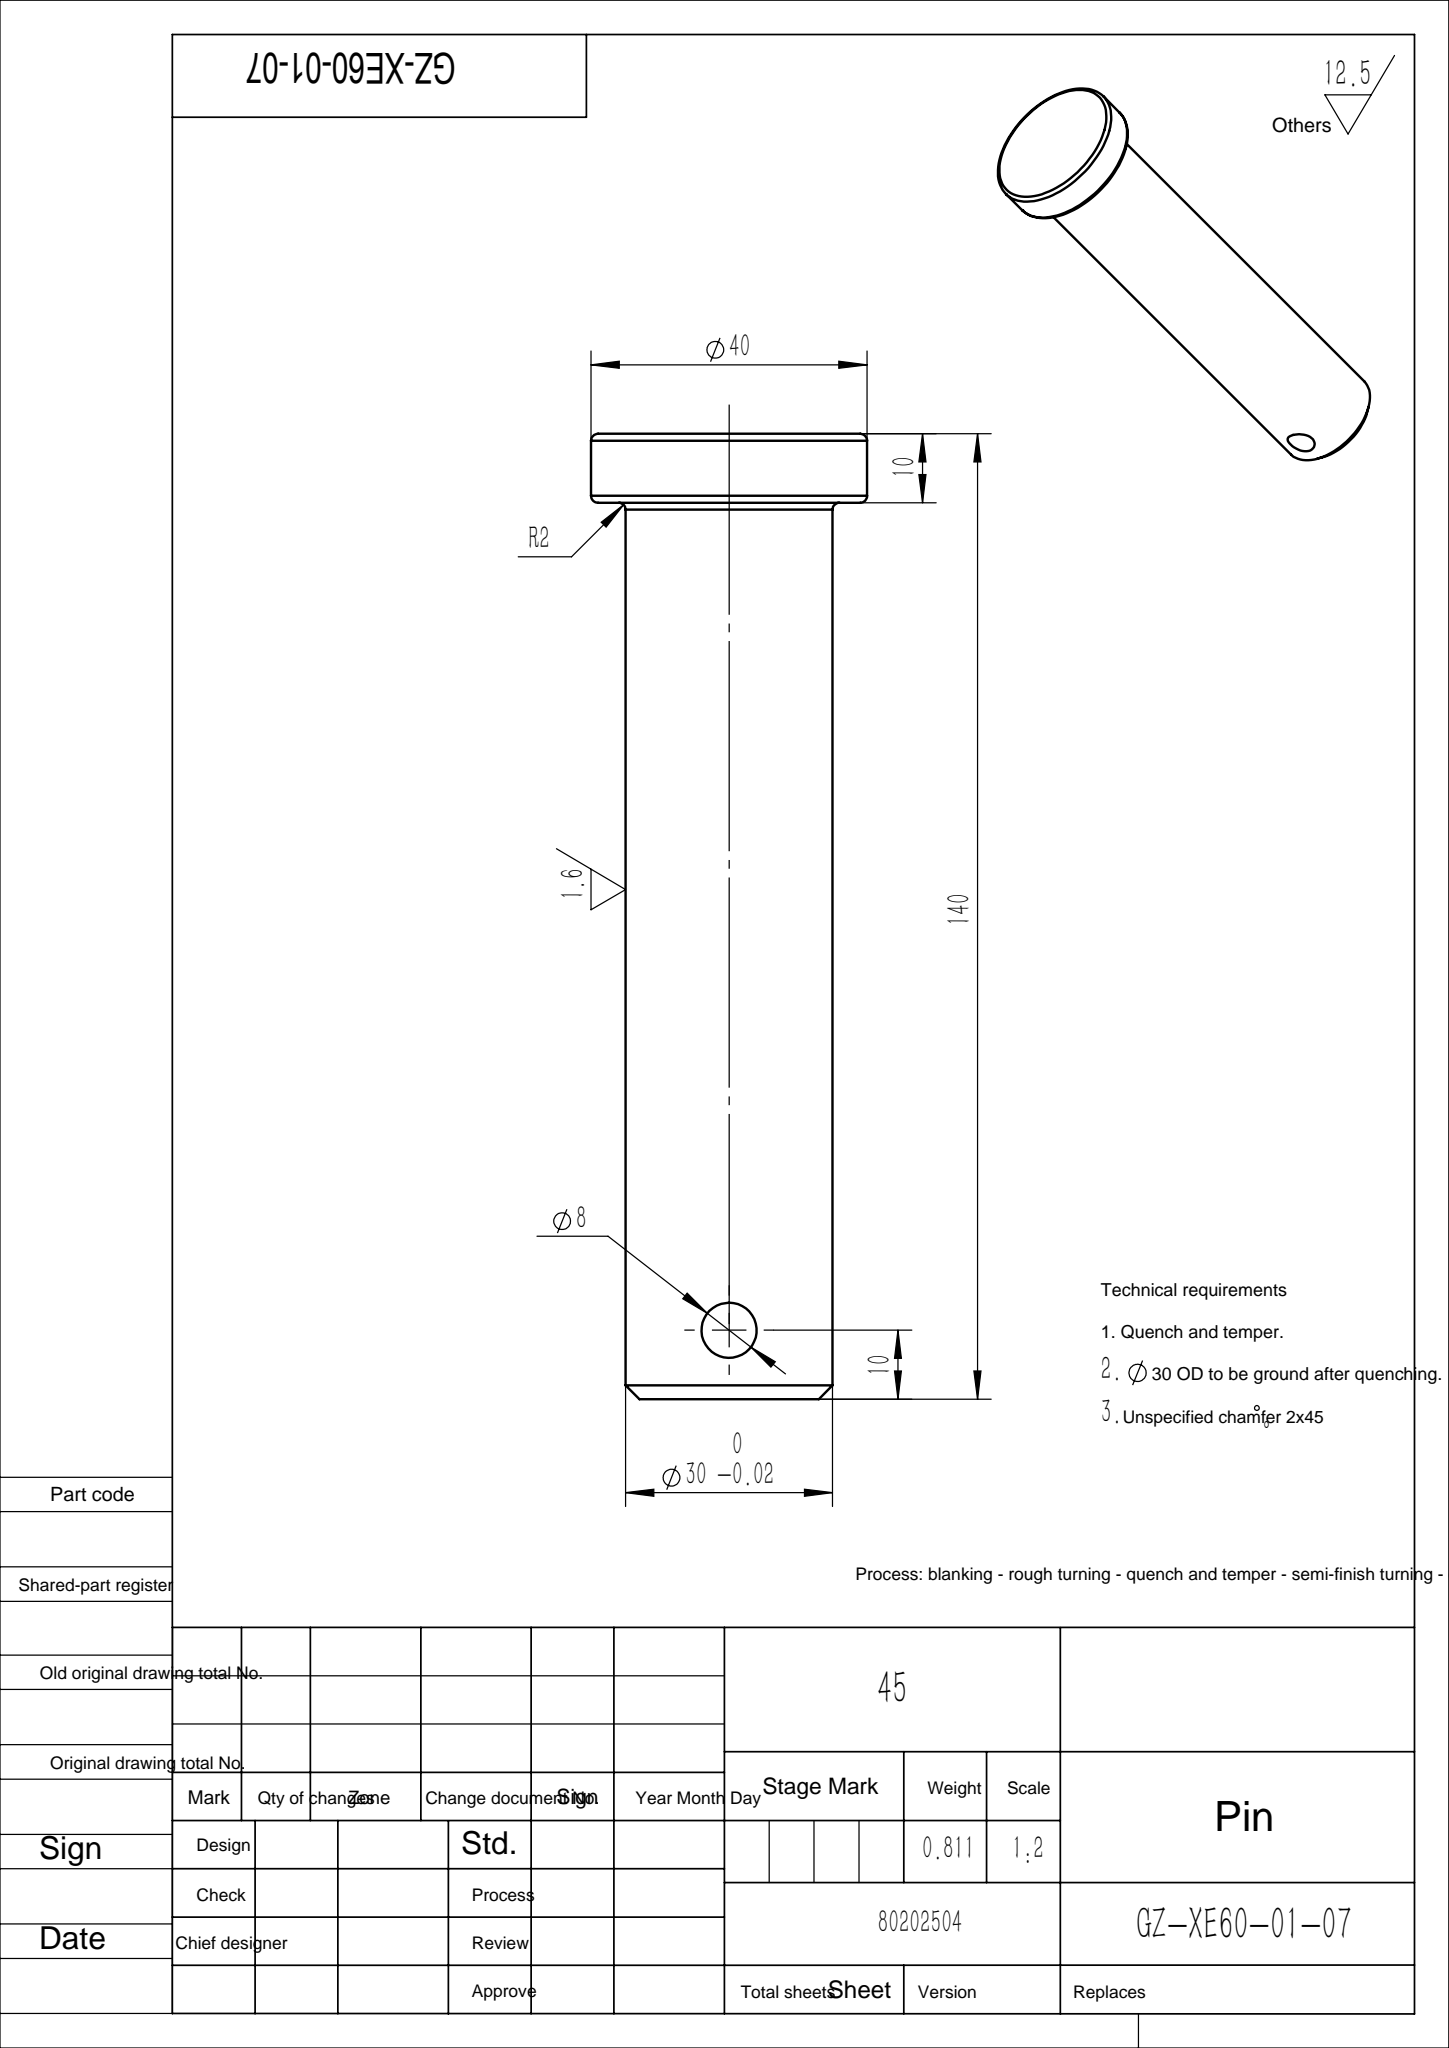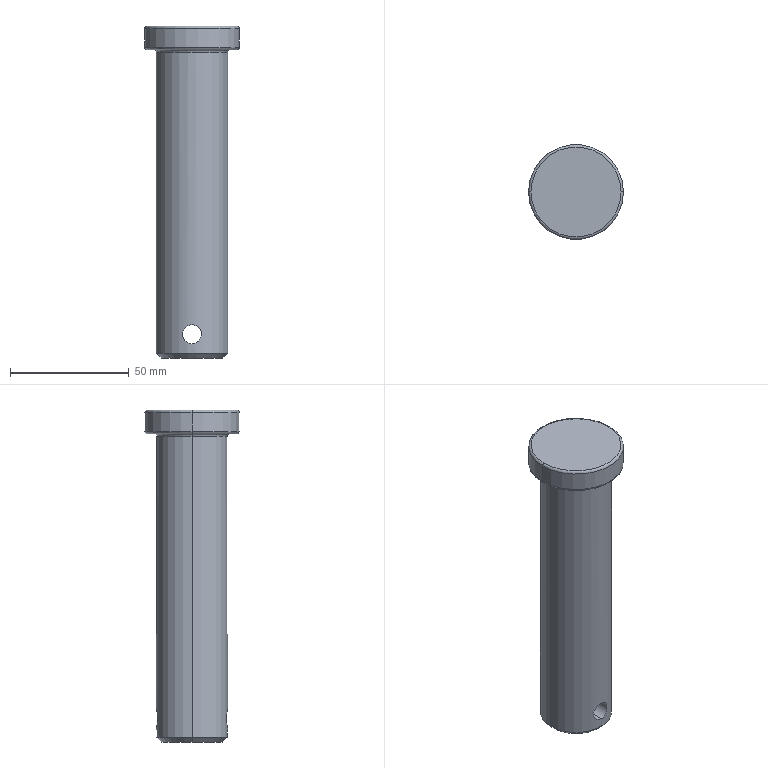Part | SolidWorks | features Fillet 2, ICE 2, Chamfer 1, Extrusion 1 | 1 solid | 17 faces | box 40 x 40 x 140 mm | volume 102751 mm3 | torus 6 | cylinder 6 | plane 3 | cone 2 | commonest cylinder face diameters 8 x2 30 x2 40 x2
STEP:
#1=CARTESIAN_POINT('',(-20.,0.,139.));
#2=VERTEX_POINT('',#1);
#3=CARTESIAN_POINT('',(20.,0.,139.));
#4=VERTEX_POINT('',#3);
#5=CARTESIAN_POINT('',(0.,0.,139.));
#6=DIRECTION('',(0.,0.,-1.));
#7=DIRECTION('',(1.,0.,0.));
#8=AXIS2_PLACEMENT_3D('',#5,#6,#7);
#9=CIRCLE('',#8,20.);
#10=EDGE_CURVE('',#2,#4,#9,.T.);
#11=ORIENTED_EDGE('',*,*,#10,.F.);
#12=CARTESIAN_POINT('',(-19.,0.,140.));
#13=VERTEX_POINT('',#12);
#14=CARTESIAN_POINT('',(-19.,0.,139.));
#15=DIRECTION('',(0.,1.,0.));
#16=DIRECTION('',(-1.,0.,0.));
#17=AXIS2_PLACEMENT_3D('',#14,#15,#16);
#18=CIRCLE('',#17,1.);
#19=EDGE_CURVE('',#2,#13,#18,.T.);
#20=ORIENTED_EDGE('',*,*,#19,.T.);
#21=CARTESIAN_POINT('',(19.,0.,140.));
#22=VERTEX_POINT('',#21);
#23=CARTESIAN_POINT('',(0.,0.,140.));
#24=DIRECTION('',(0.,0.,1.));
#25=DIRECTION('',(1.,0.,0.));
#26=AXIS2_PLACEMENT_3D('',#23,#24,#25);
#27=CIRCLE('',#26,19.);
#28=EDGE_CURVE('',#22,#13,#27,.T.);
#29=ORIENTED_EDGE('',*,*,#28,.F.);
#30=CARTESIAN_POINT('',(19.,0.,139.));
#31=DIRECTION('',(0.,-1.,0.));
#32=DIRECTION('',(0.,0.,-1.));
#33=AXIS2_PLACEMENT_3D('',#30,#31,#32);
#34=CIRCLE('',#33,1.);
#35=EDGE_CURVE('',#4,#22,#34,.T.);
#36=ORIENTED_EDGE('',*,*,#35,.F.);
#37=EDGE_LOOP('',(#11,#20,#29,#36));
#38=FACE_OUTER_BOUND('',#37,.T.);
#39=CARTESIAN_POINT('',(0.,0.,139.));
#40=DIRECTION('',(0.,0.,1.));
#41=DIRECTION('',(1.,0.,0.));
#42=AXIS2_PLACEMENT_3D('',#39,#40,#41);
#43=TOROIDAL_SURFACE('',#42,19.,1.);
#44=ADVANCED_FACE('',(#38),#43,.T.);
#45=CARTESIAN_POINT('',(-19.,0.,130.));
#46=VERTEX_POINT('',#45);
#47=CARTESIAN_POINT('',(19.,0.,130.));
#48=VERTEX_POINT('',#47);
#49=CARTESIAN_POINT('',(0.,0.,130.));
#50=DIRECTION('',(0.,0.,-1.));
#51=DIRECTION('',(1.,0.,0.));
#52=AXIS2_PLACEMENT_3D('',#49,#50,#51);
#53=CIRCLE('',#52,19.);
#54=EDGE_CURVE('',#46,#48,#53,.T.);
#55=ORIENTED_EDGE('',*,*,#54,.F.);
#56=CARTESIAN_POINT('',(-20.,0.,131.));
#57=VERTEX_POINT('',#56);
#58=CARTESIAN_POINT('',(-19.,0.,131.));
#59=DIRECTION('',(0.,1.,0.));
#60=DIRECTION('',(-1.,0.,0.));
#61=AXIS2_PLACEMENT_3D('',#58,#59,#60);
#62=CIRCLE('',#61,1.);
#63=EDGE_CURVE('',#46,#57,#62,.T.);
#64=ORIENTED_EDGE('',*,*,#63,.T.);
#65=CARTESIAN_POINT('',(20.,0.,131.));
#66=VERTEX_POINT('',#65);
#67=CARTESIAN_POINT('',(0.,0.,131.));
#68=DIRECTION('',(0.,0.,1.));
#69=DIRECTION('',(1.,0.,0.));
#70=AXIS2_PLACEMENT_3D('',#67,#68,#69);
#71=CIRCLE('',#70,20.);
#72=EDGE_CURVE('',#66,#57,#71,.T.);
#73=ORIENTED_EDGE('',*,*,#72,.F.);
#74=CARTESIAN_POINT('',(19.,0.,131.));
#75=DIRECTION('',(0.,-1.,0.));
#76=DIRECTION('',(0.,0.,-1.));
#77=AXIS2_PLACEMENT_3D('',#74,#75,#76);
#78=CIRCLE('',#77,1.);
#79=EDGE_CURVE('',#48,#66,#78,.T.);
#80=ORIENTED_EDGE('',*,*,#79,.F.);
#81=EDGE_LOOP('',(#55,#64,#73,#80));
#82=FACE_OUTER_BOUND('',#81,.T.);
#83=CARTESIAN_POINT('',(0.,0.,131.));
#84=DIRECTION('',(0.,0.,1.));
#85=DIRECTION('',(1.,0.,0.));
#86=AXIS2_PLACEMENT_3D('',#83,#84,#85);
#87=TOROIDAL_SURFACE('',#86,19.,1.);
#88=ADVANCED_FACE('',(#82),#87,.T.);
#89=CARTESIAN_POINT('',(-16.,0.,130.));
#90=VERTEX_POINT('',#89);
#91=CARTESIAN_POINT('',(16.,0.,130.));
#92=VERTEX_POINT('',#91);
#93=CARTESIAN_POINT('',(0.,0.,130.));
#94=DIRECTION('',(0.,0.,1.));
#95=DIRECTION('',(1.,0.,0.));
#96=AXIS2_PLACEMENT_3D('',#93,#94,#95);
#97=CIRCLE('',#96,16.);
#98=EDGE_CURVE('',#90,#92,#97,.T.);
#99=ORIENTED_EDGE('',*,*,#98,.F.);
#100=CARTESIAN_POINT('',(-15.,0.,129.));
#101=VERTEX_POINT('',#100);
#102=CARTESIAN_POINT('',(-16.,0.,129.));
#103=DIRECTION('',(0.,1.,0.));
#104=DIRECTION('',(-1.,0.,0.));
#105=AXIS2_PLACEMENT_3D('',#102,#103,#104);
#106=CIRCLE('',#105,1.);
#107=EDGE_CURVE('',#90,#101,#106,.T.);
#108=ORIENTED_EDGE('',*,*,#107,.T.);
#109=CARTESIAN_POINT('',(15.,0.,129.));
#110=VERTEX_POINT('',#109);
#111=CARTESIAN_POINT('',(0.,0.,129.));
#112=DIRECTION('',(0.,0.,-1.));
#113=DIRECTION('',(1.,0.,0.));
#114=AXIS2_PLACEMENT_3D('',#111,#112,#113);
#115=CIRCLE('',#114,15.);
#116=EDGE_CURVE('',#110,#101,#115,.T.);
#117=ORIENTED_EDGE('',*,*,#116,.F.);
#118=CARTESIAN_POINT('',(16.,0.,129.));
#119=DIRECTION('',(0.,-1.,0.));
#120=DIRECTION('',(0.,0.,-1.));
#121=AXIS2_PLACEMENT_3D('',#118,#119,#120);
#122=CIRCLE('',#121,1.);
#123=EDGE_CURVE('',#92,#110,#122,.T.);
#124=ORIENTED_EDGE('',*,*,#123,.F.);
#125=EDGE_LOOP('',(#99,#108,#117,#124));
#126=FACE_OUTER_BOUND('',#125,.T.);
#127=CARTESIAN_POINT('',(0.,0.,129.));
#128=DIRECTION('',(0.,0.,1.));
#129=DIRECTION('',(1.,0.,0.));
#130=AXIS2_PLACEMENT_3D('',#127,#128,#129);
#131=TOROIDAL_SURFACE('',#130,16.,1.);
#132=ADVANCED_FACE('',(#126),#131,.F.);
#133=CARTESIAN_POINT('',(-13.,0.,0.));
#134=VERTEX_POINT('',#133);
#135=CARTESIAN_POINT('',(13.,0.,0.));
#136=VERTEX_POINT('',#135);
#137=CARTESIAN_POINT('',(0.,0.,0.));
#138=DIRECTION('',(0.,0.,-1.));
#139=DIRECTION('',(1.,0.,0.));
#140=AXIS2_PLACEMENT_3D('',#137,#138,#139);
#141=CIRCLE('',#140,13.);
#142=EDGE_CURVE('',#134,#136,#141,.T.);
#143=ORIENTED_EDGE('',*,*,#142,.F.);
#144=CARTESIAN_POINT('',(-15.,0.,2.));
#145=VERTEX_POINT('',#144);
#146=CARTESIAN_POINT('',(-15.,0.,2.));
#147=DIRECTION('',(-0.7071,0.,0.7071));
#148=VECTOR('',#147,1000.);
#149=LINE('',#146,#148);
#150=EDGE_CURVE('',#134,#145,#149,.T.);
#151=ORIENTED_EDGE('',*,*,#150,.T.);
#152=CARTESIAN_POINT('',(15.,0.,2.));
#153=VERTEX_POINT('',#152);
#154=CARTESIAN_POINT('',(0.,0.,2.));
#155=DIRECTION('',(0.,0.,1.));
#156=DIRECTION('',(1.,0.,0.));
#157=AXIS2_PLACEMENT_3D('',#154,#155,#156);
#158=CIRCLE('',#157,15.);
#159=EDGE_CURVE('',#153,#145,#158,.T.);
#160=ORIENTED_EDGE('',*,*,#159,.F.);
#161=CARTESIAN_POINT('',(15.,0.,2.));
#162=DIRECTION('',(0.7071,0.,0.7071));
#163=VECTOR('',#162,1000.);
#164=LINE('',#161,#163);
#165=EDGE_CURVE('',#136,#153,#164,.T.);
#166=ORIENTED_EDGE('',*,*,#165,.F.);
#167=EDGE_LOOP('',(#143,#151,#160,#166));
#168=FACE_OUTER_BOUND('',#167,.T.);
#169=CARTESIAN_POINT('',(0.,0.,2.));
#170=DIRECTION('',(0.,0.,1.));
#171=DIRECTION('',(1.,0.,0.));
#172=AXIS2_PLACEMENT_3D('',#169,#170,#171);
#173=CONICAL_SURFACE('',#172,15.,0.7854);
#174=ADVANCED_FACE('',(#168),#173,.T.);
#175=CARTESIAN_POINT('',(0.,-15.,6.));
#176=VERTEX_POINT('',#175);
#177=CARTESIAN_POINT('',(0.,-15.,14.));
#178=VERTEX_POINT('',#177);
#179=CARTESIAN_POINT('',(0.,-15.,6.));
#180=CARTESIAN_POINT('',(-0.2617,-15.,6.));
#181=CARTESIAN_POINT('',(-0.5231,-14.993,6.026));
#182=CARTESIAN_POINT('',(-1.043,-14.966,6.129));
#183=CARTESIAN_POINT('',(-1.293,-14.946,6.206));
#184=CARTESIAN_POINT('',(-1.775,-14.897,6.406));
#185=CARTESIAN_POINT('',(-2.009,-14.866,6.531));
#186=CARTESIAN_POINT('',(-2.442,-14.801,6.822));
#187=CARTESIAN_POINT('',(-2.643,-14.767,6.986));
#188=CARTESIAN_POINT('',(-3.012,-14.696,7.355));
#189=CARTESIAN_POINT('',(-3.18,-14.66,7.559));
#190=CARTESIAN_POINT('',(-3.469,-14.594,7.991));
#191=CARTESIAN_POINT('',(-3.592,-14.564,8.22));
#192=CARTESIAN_POINT('',(-3.795,-14.512,8.707));
#193=CARTESIAN_POINT('',(-3.871,-14.492,8.959));
#194=CARTESIAN_POINT('',(-3.973,-14.464,9.471));
#195=CARTESIAN_POINT('',(-4.,-14.457,9.735));
#196=CARTESIAN_POINT('',(-4.,-14.457,10.263));
#197=CARTESIAN_POINT('',(-3.974,-14.464,10.523));
#198=CARTESIAN_POINT('',(-3.872,-14.492,11.037));
#199=CARTESIAN_POINT('',(-3.794,-14.513,11.293));
#200=CARTESIAN_POINT('',(-3.594,-14.563,11.775));
#201=CARTESIAN_POINT('',(-3.471,-14.594,12.005));
#202=CARTESIAN_POINT('',(-3.18,-14.66,12.441));
#203=CARTESIAN_POINT('',(-3.013,-14.695,12.643));
#204=CARTESIAN_POINT('',(-2.647,-14.766,13.01));
#205=CARTESIAN_POINT('',(-2.443,-14.801,13.178));
#206=CARTESIAN_POINT('',(-2.008,-14.867,13.469));
#207=CARTESIAN_POINT('',(-1.779,-14.896,13.592));
#208=CARTESIAN_POINT('',(-1.297,-14.946,13.793));
#209=CARTESIAN_POINT('',(-1.042,-14.966,13.871));
#210=CARTESIAN_POINT('',(-0.527,-14.993,13.974));
#211=CARTESIAN_POINT('',(-0.2655,-15.,14.));
#212=CARTESIAN_POINT('',(0.,-15.,14.));
#213=B_SPLINE_CURVE_WITH_KNOTS('',3,(#179,#180,#181,#182,#183,#184,#185,#186,#187,#188,#189,#190,#191,#192,#193,#194,#195,#196,#197,#198,#199,#200,#201,#202,#203,#204,#205,#206,#207,#208,#209,#210,#211,#212),.UNSPECIFIED.,.F.,.F.,(4,2,2,2,2,2,2,2,2,2,2,2,2,2,2,2,4),(0.01256,0.01335,0.01413,0.01492,0.0157,0.01649,0.01727,0.01806,0.01884,0.01963,0.02041,0.0212,0.02198,0.02277,0.02355,0.02434,0.02512),.UNSPECIFIED.);
#214=EDGE_CURVE('',#176,#178,#213,.T.);
#215=ORIENTED_EDGE('',*,*,#214,.F.);
#216=CARTESIAN_POINT('',(0.,15.,6.));
#217=VERTEX_POINT('',#216);
#218=CARTESIAN_POINT('',(0.,-20.,6.));
#219=DIRECTION('',(0.,1.,0.));
#220=VECTOR('',#219,1000.);
#221=LINE('',#218,#220);
#222=EDGE_CURVE('',#176,#217,#221,.T.);
#223=ORIENTED_EDGE('',*,*,#222,.T.);
#224=CARTESIAN_POINT('',(0.,15.,14.));
#225=VERTEX_POINT('',#224);
#226=CARTESIAN_POINT('',(0.,15.,14.));
#227=CARTESIAN_POINT('',(-0.2656,15.,14.));
#228=CARTESIAN_POINT('',(-0.5265,14.993,13.974));
#229=CARTESIAN_POINT('',(-1.039,14.966,13.871));
#230=CARTESIAN_POINT('',(-1.294,14.946,13.794));
#231=CARTESIAN_POINT('',(-1.778,14.896,13.593));
#232=CARTESIAN_POINT('',(-2.007,14.867,13.47));
#233=CARTESIAN_POINT('',(-2.441,14.802,13.179));
#234=CARTESIAN_POINT('',(-2.646,14.766,13.011));
#235=CARTESIAN_POINT('',(-3.013,14.695,12.644));
#236=CARTESIAN_POINT('',(-3.178,14.66,12.443));
#237=CARTESIAN_POINT('',(-3.47,14.594,12.006));
#238=CARTESIAN_POINT('',(-3.594,14.563,11.775));
#239=CARTESIAN_POINT('',(-3.794,14.513,11.295));
#240=CARTESIAN_POINT('',(-3.871,14.492,11.041));
#241=CARTESIAN_POINT('',(-3.974,14.464,10.524));
#242=CARTESIAN_POINT('',(-4.,14.457,10.264));
#243=CARTESIAN_POINT('',(-4.,14.457,9.739));
#244=CARTESIAN_POINT('',(-3.974,14.464,9.473));
#245=CARTESIAN_POINT('',(-3.871,14.492,8.959));
#246=CARTESIAN_POINT('',(-3.795,14.512,8.709));
#247=CARTESIAN_POINT('',(-3.493,14.589,7.98));
#248=CARTESIAN_POINT('',(-3.198,14.66,7.541));
#249=CARTESIAN_POINT('',(-2.643,14.767,6.986));
#250=CARTESIAN_POINT('',(-2.442,14.802,6.821));
#251=CARTESIAN_POINT('',(-2.01,14.866,6.532));
#252=CARTESIAN_POINT('',(-1.775,14.897,6.406));
#253=CARTESIAN_POINT('',(-1.292,14.946,6.206));
#254=CARTESIAN_POINT('',(-1.043,14.966,6.129));
#255=CARTESIAN_POINT('',(-0.5273,14.993,6.026));
#256=CARTESIAN_POINT('',(-0.2618,15.,6.));
#257=CARTESIAN_POINT('',(0.,15.,6.));
#258=B_SPLINE_CURVE_WITH_KNOTS('',3,(#226,#227,#228,#229,#230,#231,#232,#233,#234,#235,#236,#237,#238,#239,#240,#241,#242,#243,#244,#245,#246,#247,#248,#249,#250,#251,#252,#253,#254,#255,#256,#257),.UNSPECIFIED.,.F.,.F.,(4,2,2,2,2,2,2,2,2,2,2,2,2,2,2,4),(0.,0.0007852,0.00157,0.002356,0.003141,0.003926,0.004711,0.005496,0.006281,0.007067,0.007852,0.009422,0.01021,0.01099,0.01178,0.01256),.UNSPECIFIED.);
#259=EDGE_CURVE('',#225,#217,#258,.T.);
#260=ORIENTED_EDGE('',*,*,#259,.F.);
#261=CARTESIAN_POINT('',(0.,-20.,14.));
#262=DIRECTION('',(0.,1.,0.));
#263=VECTOR('',#262,1000.);
#264=LINE('',#261,#263);
#265=EDGE_CURVE('',#178,#225,#264,.T.);
#266=ORIENTED_EDGE('',*,*,#265,.F.);
#267=EDGE_LOOP('',(#215,#223,#260,#266));
#268=FACE_OUTER_BOUND('',#267,.T.);
#269=CARTESIAN_POINT('',(0.,-20.,10.));
#270=DIRECTION('',(0.,1.,0.));
#271=DIRECTION('',(0.,0.,1.));
#272=AXIS2_PLACEMENT_3D('',#269,#270,#271);
#273=CYLINDRICAL_SURFACE('',#272,4.);
#274=ADVANCED_FACE('',(#268),#273,.F.);
#275=ORIENTED_EDGE('',*,*,#10,.T.);
#276=CARTESIAN_POINT('',(20.,0.,140.));
#277=DIRECTION('',(0.,0.,-1.));
#278=VECTOR('',#277,1000.);
#279=LINE('',#276,#278);
#280=EDGE_CURVE('',#4,#66,#279,.T.);
#281=ORIENTED_EDGE('',*,*,#280,.T.);
#282=ORIENTED_EDGE('',*,*,#72,.T.);
#283=CARTESIAN_POINT('',(-20.,0.,140.));
#284=DIRECTION('',(0.,0.,-1.));
#285=VECTOR('',#284,1000.);
#286=LINE('',#283,#285);
#287=EDGE_CURVE('',#2,#57,#286,.T.);
#288=ORIENTED_EDGE('',*,*,#287,.F.);
#289=EDGE_LOOP('',(#275,#281,#282,#288));
#290=FACE_OUTER_BOUND('',#289,.T.);
#291=CARTESIAN_POINT('',(0.,0.,140.));
#292=DIRECTION('',(0.,0.,-1.));
#293=DIRECTION('',(-1.,0.,0.));
#294=AXIS2_PLACEMENT_3D('',#291,#292,#293);
#295=CYLINDRICAL_SURFACE('',#294,20.);
#296=ADVANCED_FACE('',(#290),#295,.T.);
#297=ORIENTED_EDGE('',*,*,#259,.T.);
#298=CARTESIAN_POINT('',(0.,15.,6.));
#299=CARTESIAN_POINT('',(0.2617,15.,6.));
#300=CARTESIAN_POINT('',(0.5231,14.993,6.026));
#301=CARTESIAN_POINT('',(1.043,14.966,6.129));
#302=CARTESIAN_POINT('',(1.293,14.946,6.206));
#303=CARTESIAN_POINT('',(1.775,14.897,6.406));
#304=CARTESIAN_POINT('',(2.009,14.866,6.531));
#305=CARTESIAN_POINT('',(2.442,14.801,6.822));
#306=CARTESIAN_POINT('',(2.643,14.767,6.986));
#307=CARTESIAN_POINT('',(3.012,14.696,7.355));
#308=CARTESIAN_POINT('',(3.18,14.66,7.559));
#309=CARTESIAN_POINT('',(3.469,14.594,7.991));
#310=CARTESIAN_POINT('',(3.592,14.564,8.22));
#311=CARTESIAN_POINT('',(3.795,14.512,8.707));
#312=CARTESIAN_POINT('',(3.871,14.492,8.959));
#313=CARTESIAN_POINT('',(3.973,14.464,9.471));
#314=CARTESIAN_POINT('',(4.,14.457,9.735));
#315=CARTESIAN_POINT('',(4.,14.457,10.263));
#316=CARTESIAN_POINT('',(3.974,14.464,10.523));
#317=CARTESIAN_POINT('',(3.872,14.492,11.037));
#318=CARTESIAN_POINT('',(3.794,14.513,11.293));
#319=CARTESIAN_POINT('',(3.594,14.563,11.775));
#320=CARTESIAN_POINT('',(3.471,14.594,12.005));
#321=CARTESIAN_POINT('',(3.18,14.66,12.441));
#322=CARTESIAN_POINT('',(3.013,14.695,12.643));
#323=CARTESIAN_POINT('',(2.647,14.766,13.01));
#324=CARTESIAN_POINT('',(2.443,14.801,13.178));
#325=CARTESIAN_POINT('',(2.008,14.867,13.469));
#326=CARTESIAN_POINT('',(1.779,14.896,13.592));
#327=CARTESIAN_POINT('',(1.297,14.946,13.793));
#328=CARTESIAN_POINT('',(1.042,14.966,13.871));
#329=CARTESIAN_POINT('',(0.527,14.993,13.974));
#330=CARTESIAN_POINT('',(0.2655,15.,14.));
#331=CARTESIAN_POINT('',(0.,15.,14.));
#332=B_SPLINE_CURVE_WITH_KNOTS('',3,(#298,#299,#300,#301,#302,#303,#304,#305,#306,#307,#308,#309,#310,#311,#312,#313,#314,#315,#316,#317,#318,#319,#320,#321,#322,#323,#324,#325,#326,#327,#328,#329,#330,#331),.UNSPECIFIED.,.F.,.F.,(4,2,2,2,2,2,2,2,2,2,2,2,2,2,2,2,4),(0.01256,0.01335,0.01413,0.01492,0.0157,0.01649,0.01727,0.01806,0.01884,0.01963,0.02041,0.0212,0.02198,0.02277,0.02355,0.02434,0.02512),.UNSPECIFIED.);
#333=EDGE_CURVE('',#217,#225,#332,.T.);
#334=ORIENTED_EDGE('',*,*,#333,.T.);
#335=EDGE_LOOP('',(#297,#334));
#336=FACE_BOUND('',#335,.T.);
#337=CARTESIAN_POINT('',(0.,0.,129.));
#338=DIRECTION('',(0.,0.,-1.));
#339=DIRECTION('',(1.,0.,0.));
#340=AXIS2_PLACEMENT_3D('',#337,#338,#339);
#341=CIRCLE('',#340,15.);
#342=EDGE_CURVE('',#101,#110,#341,.T.);
#343=ORIENTED_EDGE('',*,*,#342,.T.);
#344=CARTESIAN_POINT('',(15.,0.,130.));
#345=DIRECTION('',(0.,0.,-1.));
#346=VECTOR('',#345,1000.);
#347=LINE('',#344,#346);
#348=EDGE_CURVE('',#110,#153,#347,.T.);
#349=ORIENTED_EDGE('',*,*,#348,.T.);
#350=ORIENTED_EDGE('',*,*,#159,.T.);
#351=CARTESIAN_POINT('',(-15.,0.,130.));
#352=DIRECTION('',(0.,0.,-1.));
#353=VECTOR('',#352,1000.);
#354=LINE('',#351,#353);
#355=EDGE_CURVE('',#101,#145,#354,.T.);
#356=ORIENTED_EDGE('',*,*,#355,.F.);
#357=EDGE_LOOP('',(#343,#349,#350,#356));
#358=FACE_OUTER_BOUND('',#357,.T.);
#359=CARTESIAN_POINT('',(0.,0.,130.));
#360=DIRECTION('',(0.,0.,-1.));
#361=DIRECTION('',(-1.,0.,0.));
#362=AXIS2_PLACEMENT_3D('',#359,#360,#361);
#363=CYLINDRICAL_SURFACE('',#362,15.);
#364=ADVANCED_FACE('',(#336,#358),#363,.T.);
#365=ORIENTED_EDGE('',*,*,#348,.F.);
#366=ORIENTED_EDGE('',*,*,#116,.T.);
#367=ORIENTED_EDGE('',*,*,#355,.T.);
#368=CARTESIAN_POINT('',(0.,0.,2.));
#369=DIRECTION('',(0.,0.,1.));
#370=DIRECTION('',(1.,0.,0.));
#371=AXIS2_PLACEMENT_3D('',#368,#369,#370);
#372=CIRCLE('',#371,15.);
#373=EDGE_CURVE('',#145,#153,#372,.T.);
#374=ORIENTED_EDGE('',*,*,#373,.T.);
#375=EDGE_LOOP('',(#365,#366,#367,#374));
#376=FACE_OUTER_BOUND('',#375,.T.);
#377=CARTESIAN_POINT('',(0.,-15.,14.));
#378=CARTESIAN_POINT('',(0.2656,-15.,14.));
#379=CARTESIAN_POINT('',(0.5265,-14.993,13.974));
#380=CARTESIAN_POINT('',(1.039,-14.966,13.871));
#381=CARTESIAN_POINT('',(1.294,-14.946,13.794));
#382=CARTESIAN_POINT('',(1.778,-14.896,13.593));
#383=CARTESIAN_POINT('',(2.007,-14.867,13.47));
#384=CARTESIAN_POINT('',(2.441,-14.802,13.179));
#385=CARTESIAN_POINT('',(2.646,-14.766,13.011));
#386=CARTESIAN_POINT('',(3.013,-14.695,12.644));
#387=CARTESIAN_POINT('',(3.178,-14.66,12.443));
#388=CARTESIAN_POINT('',(3.47,-14.594,12.006));
#389=CARTESIAN_POINT('',(3.594,-14.563,11.775));
#390=CARTESIAN_POINT('',(3.794,-14.513,11.295));
#391=CARTESIAN_POINT('',(3.871,-14.492,11.041));
#392=CARTESIAN_POINT('',(3.974,-14.464,10.524));
#393=CARTESIAN_POINT('',(4.,-14.457,10.264));
#394=CARTESIAN_POINT('',(4.,-14.457,9.739));
#395=CARTESIAN_POINT('',(3.974,-14.464,9.473));
#396=CARTESIAN_POINT('',(3.871,-14.492,8.959));
#397=CARTESIAN_POINT('',(3.795,-14.512,8.709));
#398=CARTESIAN_POINT('',(3.493,-14.589,7.98));
#399=CARTESIAN_POINT('',(3.198,-14.66,7.541));
#400=CARTESIAN_POINT('',(2.643,-14.767,6.986));
#401=CARTESIAN_POINT('',(2.442,-14.802,6.821));
#402=CARTESIAN_POINT('',(2.01,-14.866,6.532));
#403=CARTESIAN_POINT('',(1.775,-14.897,6.406));
#404=CARTESIAN_POINT('',(1.292,-14.946,6.206));
#405=CARTESIAN_POINT('',(1.043,-14.966,6.129));
#406=CARTESIAN_POINT('',(0.5273,-14.993,6.026));
#407=CARTESIAN_POINT('',(0.2618,-15.,6.));
#408=CARTESIAN_POINT('',(0.,-15.,6.));
#409=B_SPLINE_CURVE_WITH_KNOTS('',3,(#377,#378,#379,#380,#381,#382,#383,#384,#385,#386,#387,#388,#389,#390,#391,#392,#393,#394,#395,#396,#397,#398,#399,#400,#401,#402,#403,#404,#405,#406,#407,#408),.UNSPECIFIED.,.F.,.F.,(4,2,2,2,2,2,2,2,2,2,2,2,2,2,2,4),(0.,0.0007852,0.00157,0.002356,0.003141,0.003926,0.004711,0.005496,0.006281,0.007067,0.007852,0.009422,0.01021,0.01099,0.01178,0.01256),.UNSPECIFIED.);
#410=EDGE_CURVE('',#178,#176,#409,.T.);
#411=ORIENTED_EDGE('',*,*,#410,.T.);
#412=ORIENTED_EDGE('',*,*,#214,.T.);
#413=EDGE_LOOP('',(#411,#412));
#414=FACE_BOUND('',#413,.T.);
#415=CARTESIAN_POINT('',(0.,0.,130.));
#416=DIRECTION('',(0.,0.,-1.));
#417=DIRECTION('',(-1.,0.,0.));
#418=AXIS2_PLACEMENT_3D('',#415,#416,#417);
#419=CYLINDRICAL_SURFACE('',#418,15.);
#420=ADVANCED_FACE('',(#376,#414),#419,.T.);
#421=CARTESIAN_POINT('',(0.,0.,0.));
#422=DIRECTION('',(0.,0.,-1.));
#423=DIRECTION('',(1.,0.,0.));
#424=AXIS2_PLACEMENT_3D('',#421,#422,#423);
#425=CIRCLE('',#424,13.);
#426=EDGE_CURVE('',#136,#134,#425,.T.);
#427=ORIENTED_EDGE('',*,*,#426,.T.);
#428=ORIENTED_EDGE('',*,*,#142,.T.);
#429=EDGE_LOOP('',(#427,#428));
#430=FACE_OUTER_BOUND('',#429,.T.);
#431=CARTESIAN_POINT('',(0.,0.,0.));
#432=DIRECTION('',(0.,0.,1.));
#433=DIRECTION('',(1.,0.,0.));
#434=AXIS2_PLACEMENT_3D('',#431,#432,#433);
#435=PLANE('',#434);
#436=ADVANCED_FACE('',(#430),#435,.F.);
#437=ORIENTED_EDGE('',*,*,#280,.F.);
#438=CARTESIAN_POINT('',(0.,0.,139.));
#439=DIRECTION('',(0.,0.,-1.));
#440=DIRECTION('',(1.,0.,0.));
#441=AXIS2_PLACEMENT_3D('',#438,#439,#440);
#442=CIRCLE('',#441,20.);
#443=EDGE_CURVE('',#4,#2,#442,.T.);
#444=ORIENTED_EDGE('',*,*,#443,.T.);
#445=ORIENTED_EDGE('',*,*,#287,.T.);
#446=CARTESIAN_POINT('',(0.,0.,131.));
#447=DIRECTION('',(0.,0.,1.));
#448=DIRECTION('',(1.,0.,0.));
#449=AXIS2_PLACEMENT_3D('',#446,#447,#448);
#450=CIRCLE('',#449,20.);
#451=EDGE_CURVE('',#57,#66,#450,.T.);
#452=ORIENTED_EDGE('',*,*,#451,.T.);
#453=EDGE_LOOP('',(#437,#444,#445,#452));
#454=FACE_OUTER_BOUND('',#453,.T.);
#455=CARTESIAN_POINT('',(0.,0.,140.));
#456=DIRECTION('',(0.,0.,-1.));
#457=DIRECTION('',(-1.,0.,0.));
#458=AXIS2_PLACEMENT_3D('',#455,#456,#457);
#459=CYLINDRICAL_SURFACE('',#458,20.);
#460=ADVANCED_FACE('',(#454),#459,.T.);
#461=ORIENTED_EDGE('',*,*,#28,.T.);
#462=CARTESIAN_POINT('',(0.,0.,140.));
#463=DIRECTION('',(0.,0.,1.));
#464=DIRECTION('',(1.,0.,0.));
#465=AXIS2_PLACEMENT_3D('',#462,#463,#464);
#466=CIRCLE('',#465,19.);
#467=EDGE_CURVE('',#13,#22,#466,.T.);
#468=ORIENTED_EDGE('',*,*,#467,.T.);
#469=EDGE_LOOP('',(#461,#468));
#470=FACE_OUTER_BOUND('',#469,.T.);
#471=CARTESIAN_POINT('',(0.,0.,140.));
#472=DIRECTION('',(0.,0.,1.));
#473=DIRECTION('',(1.,0.,0.));
#474=AXIS2_PLACEMENT_3D('',#471,#472,#473);
#475=PLANE('',#474);
#476=ADVANCED_FACE('',(#470),#475,.T.);
#477=CARTESIAN_POINT('',(0.,0.,130.));
#478=DIRECTION('',(0.,0.,-1.));
#479=DIRECTION('',(1.,0.,0.));
#480=AXIS2_PLACEMENT_3D('',#477,#478,#479);
#481=CIRCLE('',#480,19.);
#482=EDGE_CURVE('',#48,#46,#481,.T.);
#483=ORIENTED_EDGE('',*,*,#482,.T.);
#484=ORIENTED_EDGE('',*,*,#54,.T.);
#485=EDGE_LOOP('',(#483,#484));
#486=FACE_OUTER_BOUND('',#485,.T.);
#487=CARTESIAN_POINT('',(0.,0.,130.));
#488=DIRECTION('',(0.,0.,1.));
#489=DIRECTION('',(1.,0.,0.));
#490=AXIS2_PLACEMENT_3D('',#487,#488,#489);
#491=CIRCLE('',#490,16.);
#492=EDGE_CURVE('',#92,#90,#491,.T.);
#493=ORIENTED_EDGE('',*,*,#492,.T.);
#494=ORIENTED_EDGE('',*,*,#98,.T.);
#495=EDGE_LOOP('',(#493,#494));
#496=FACE_BOUND('',#495,.T.);
#497=CARTESIAN_POINT('',(0.,0.,130.));
#498=DIRECTION('',(0.,0.,1.));
#499=DIRECTION('',(1.,0.,0.));
#500=AXIS2_PLACEMENT_3D('',#497,#498,#499);
#501=PLANE('',#500);
#502=ADVANCED_FACE('',(#486,#496),#501,.F.);
#503=ORIENTED_EDGE('',*,*,#222,.F.);
#504=ORIENTED_EDGE('',*,*,#410,.F.);
#505=ORIENTED_EDGE('',*,*,#265,.T.);
#506=ORIENTED_EDGE('',*,*,#333,.F.);
#507=EDGE_LOOP('',(#503,#504,#505,#506));
#508=FACE_OUTER_BOUND('',#507,.T.);
#509=CARTESIAN_POINT('',(0.,-20.,10.));
#510=DIRECTION('',(0.,1.,0.));
#511=DIRECTION('',(0.,0.,1.));
#512=AXIS2_PLACEMENT_3D('',#509,#510,#511);
#513=CYLINDRICAL_SURFACE('',#512,4.);
#514=ADVANCED_FACE('',(#508),#513,.F.);
#515=ORIENTED_EDGE('',*,*,#150,.F.);
#516=ORIENTED_EDGE('',*,*,#426,.F.);
#517=ORIENTED_EDGE('',*,*,#165,.T.);
#518=ORIENTED_EDGE('',*,*,#373,.F.);
#519=EDGE_LOOP('',(#515,#516,#517,#518));
#520=FACE_OUTER_BOUND('',#519,.T.);
#521=CARTESIAN_POINT('',(0.,0.,2.));
#522=DIRECTION('',(0.,0.,1.));
#523=DIRECTION('',(1.,0.,0.));
#524=AXIS2_PLACEMENT_3D('',#521,#522,#523);
#525=CONICAL_SURFACE('',#524,15.,0.7854);
#526=ADVANCED_FACE('',(#520),#525,.T.);
#527=ORIENTED_EDGE('',*,*,#107,.F.);
#528=ORIENTED_EDGE('',*,*,#492,.F.);
#529=ORIENTED_EDGE('',*,*,#123,.T.);
#530=ORIENTED_EDGE('',*,*,#342,.F.);
#531=EDGE_LOOP('',(#527,#528,#529,#530));
#532=FACE_OUTER_BOUND('',#531,.T.);
#533=CARTESIAN_POINT('',(0.,0.,129.));
#534=DIRECTION('',(0.,0.,1.));
#535=DIRECTION('',(1.,0.,0.));
#536=AXIS2_PLACEMENT_3D('',#533,#534,#535);
#537=TOROIDAL_SURFACE('',#536,16.,1.);
#538=ADVANCED_FACE('',(#532),#537,.F.);
#539=ORIENTED_EDGE('',*,*,#63,.F.);
#540=ORIENTED_EDGE('',*,*,#482,.F.);
#541=ORIENTED_EDGE('',*,*,#79,.T.);
#542=ORIENTED_EDGE('',*,*,#451,.F.);
#543=EDGE_LOOP('',(#539,#540,#541,#542));
#544=FACE_OUTER_BOUND('',#543,.T.);
#545=CARTESIAN_POINT('',(0.,0.,131.));
#546=DIRECTION('',(0.,0.,1.));
#547=DIRECTION('',(1.,0.,0.));
#548=AXIS2_PLACEMENT_3D('',#545,#546,#547);
#549=TOROIDAL_SURFACE('',#548,19.,1.);
#550=ADVANCED_FACE('',(#544),#549,.T.);
#551=ORIENTED_EDGE('',*,*,#19,.F.);
#552=ORIENTED_EDGE('',*,*,#443,.F.);
#553=ORIENTED_EDGE('',*,*,#35,.T.);
#554=ORIENTED_EDGE('',*,*,#467,.F.);
#555=EDGE_LOOP('',(#551,#552,#553,#554));
#556=FACE_OUTER_BOUND('',#555,.T.);
#557=CARTESIAN_POINT('',(0.,0.,139.));
#558=DIRECTION('',(0.,0.,1.));
#559=DIRECTION('',(1.,0.,0.));
#560=AXIS2_PLACEMENT_3D('',#557,#558,#559);
#561=TOROIDAL_SURFACE('',#560,19.,1.);
#562=ADVANCED_FACE('',(#556),#561,.T.);
#563=CLOSED_SHELL('',(#44,#88,#132,#174,#274,#296,#364,#420,#436,#460,#476,#502,#514,#526,#538,#550,#562));
#564=MANIFOLD_SOLID_BREP('',#563);
#565=CARTESIAN_POINT('',(0.,0.,0.));
#566=DIRECTION('',(0.,0.,1.));
#567=DIRECTION('',(1.,0.,0.));
#568=AXIS2_PLACEMENT_3D('',#565,#566,#567);
#569=(LENGTH_UNIT()NAMED_UNIT(*)SI_UNIT(.MILLI.,.METRE.));
#570=UNCERTAINTY_MEASURE_WITH_UNIT(LENGTH_MEASURE(0.00001),#569,'','');
#571=(NAMED_UNIT(*)PLANE_ANGLE_UNIT()SI_UNIT($,.RADIAN.));
#572=(NAMED_UNIT(*)SI_UNIT($,.STERADIAN.)SOLID_ANGLE_UNIT());
#573=(GEOMETRIC_REPRESENTATION_CONTEXT(3)GLOBAL_UNCERTAINTY_ASSIGNED_CONTEXT((#570))GLOBAL_UNIT_ASSIGNED_CONTEXT((#569,#571,#572))REPRESENTATION_CONTEXT('',''));
#574=ADVANCED_BREP_SHAPE_REPRESENTATION('',(#564,#568),#573);